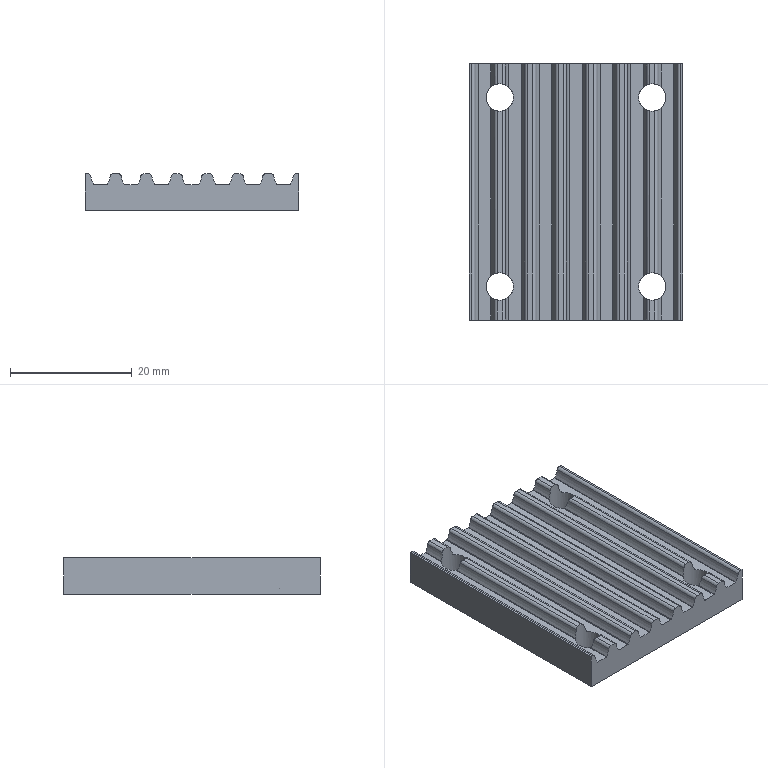Part | SolidWorks | features BaseBody 1 | 1 solid | 98 faces | box 35 x 42 x 6 mm | volume 6923 mm3 | cylinder 74 | plane 24 | commonest cylinder face diameters 0.2 x22 1 x22 6.5 x22 4.5 x8